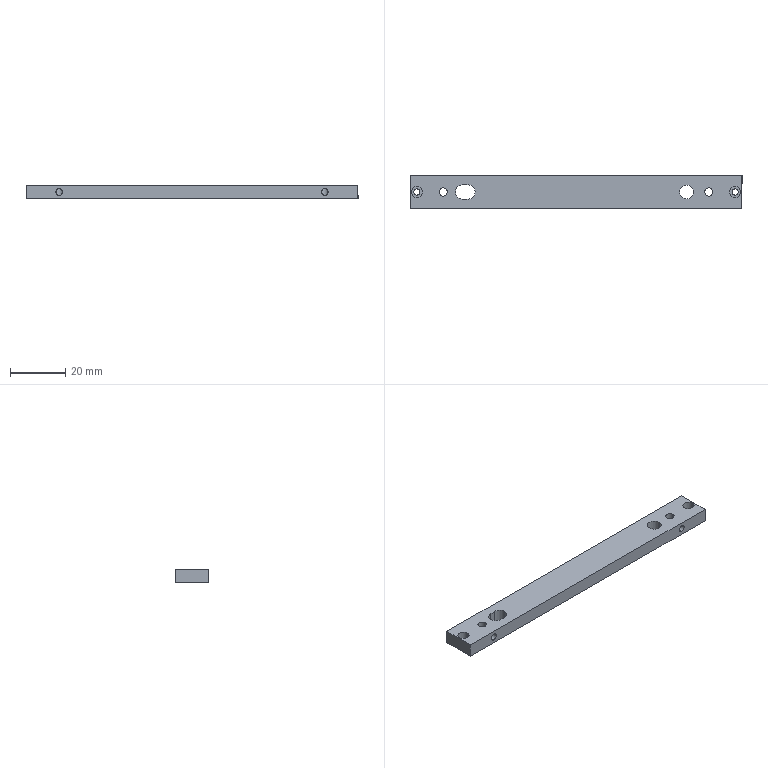Part | SolidWorks | features BaseBody 1 | 1 solid | 35 faces | box 120 x 12 x 5 mm | volume 6743 mm3 | cylinder 21 | plane 10 | cone 4 | commonest cylinder face diameters 2.2 x4 2.459 x4 3 x4 4 x4 5.1 x3 5 x2
STEP:
#1=CARTESIAN_POINT('',(-13.795,0.958,0.));
#2=VERTEX_POINT('',#1);
#3=CARTESIAN_POINT('',(-15.995,0.958,0.));
#4=VERTEX_POINT('',#3);
#5=CARTESIAN_POINT('',(-14.895,0.958,0.));
#6=DIRECTION('',(0.,0.,-1.));
#7=DIRECTION('',(1.,0.,0.));
#8=AXIS2_PLACEMENT_3D('',#5,#6,#7);
#9=CIRCLE('',#8,1.1);
#10=EDGE_CURVE('',#2,#4,#9,.T.);
#11=ORIENTED_EDGE('',*,*,#10,.T.);
#12=CARTESIAN_POINT('',(-15.995,0.958,2.));
#13=VERTEX_POINT('',#12);
#14=CARTESIAN_POINT('',(-15.995,0.958,-115.702));
#15=DIRECTION('',(0.,0.,1.));
#16=VECTOR('',#15,1000.);
#17=LINE('',#14,#16);
#18=EDGE_CURVE('',#4,#13,#17,.T.);
#19=ORIENTED_EDGE('',*,*,#18,.T.);
#20=CARTESIAN_POINT('',(-13.795,0.958,2.));
#21=VERTEX_POINT('',#20);
#22=CARTESIAN_POINT('',(-14.895,0.958,2.));
#23=DIRECTION('',(0.,0.,-1.));
#24=DIRECTION('',(1.,0.,0.));
#25=AXIS2_PLACEMENT_3D('',#22,#23,#24);
#26=CIRCLE('',#25,1.1);
#27=EDGE_CURVE('',#21,#13,#26,.T.);
#28=ORIENTED_EDGE('',*,*,#27,.F.);
#29=CARTESIAN_POINT('',(-13.795,0.958,-115.702));
#30=DIRECTION('',(0.,0.,1.));
#31=VECTOR('',#30,1000.);
#32=LINE('',#29,#31);
#33=EDGE_CURVE('',#2,#21,#32,.T.);
#34=ORIENTED_EDGE('',*,*,#33,.F.);
#35=EDGE_LOOP('',(#11,#19,#28,#34));
#36=FACE_OUTER_BOUND('',#35,.T.);
#37=CARTESIAN_POINT('',(-14.895,0.958,-115.702));
#38=DIRECTION('',(0.,0.,1.));
#39=DIRECTION('',(1.,0.,0.));
#40=AXIS2_PLACEMENT_3D('',#37,#38,#39);
#41=CYLINDRICAL_SURFACE('',#40,1.1);
#42=ADVANCED_FACE('',(#36),#41,.F.);
#43=CARTESIAN_POINT('',(101.205,0.958,0.));
#44=VERTEX_POINT('',#43);
#45=CARTESIAN_POINT('',(99.005,0.958,0.));
#46=VERTEX_POINT('',#45);
#47=CARTESIAN_POINT('',(100.105,0.958,0.));
#48=DIRECTION('',(0.,0.,-1.));
#49=DIRECTION('',(1.,0.,0.));
#50=AXIS2_PLACEMENT_3D('',#47,#48,#49);
#51=CIRCLE('',#50,1.1);
#52=EDGE_CURVE('',#44,#46,#51,.T.);
#53=ORIENTED_EDGE('',*,*,#52,.T.);
#54=CARTESIAN_POINT('',(99.005,0.958,2.));
#55=VERTEX_POINT('',#54);
#56=CARTESIAN_POINT('',(99.005,0.958,-115.702));
#57=DIRECTION('',(0.,0.,1.));
#58=VECTOR('',#57,1000.);
#59=LINE('',#56,#58);
#60=EDGE_CURVE('',#46,#55,#59,.T.);
#61=ORIENTED_EDGE('',*,*,#60,.T.);
#62=CARTESIAN_POINT('',(101.205,0.958,2.));
#63=VERTEX_POINT('',#62);
#64=CARTESIAN_POINT('',(100.105,0.958,2.));
#65=DIRECTION('',(0.,0.,-1.));
#66=DIRECTION('',(1.,0.,0.));
#67=AXIS2_PLACEMENT_3D('',#64,#65,#66);
#68=CIRCLE('',#67,1.1);
#69=EDGE_CURVE('',#63,#55,#68,.T.);
#70=ORIENTED_EDGE('',*,*,#69,.F.);
#71=CARTESIAN_POINT('',(101.205,0.958,-115.702));
#72=DIRECTION('',(0.,0.,1.));
#73=VECTOR('',#72,1000.);
#74=LINE('',#71,#73);
#75=EDGE_CURVE('',#44,#63,#74,.T.);
#76=ORIENTED_EDGE('',*,*,#75,.F.);
#77=EDGE_LOOP('',(#53,#61,#70,#76));
#78=FACE_OUTER_BOUND('',#77,.T.);
#79=CARTESIAN_POINT('',(100.105,0.958,-115.702));
#80=DIRECTION('',(0.,0.,1.));
#81=DIRECTION('',(1.,0.,0.));
#82=AXIS2_PLACEMENT_3D('',#79,#80,#81);
#83=CYLINDRICAL_SURFACE('',#82,1.1);
#84=ADVANCED_FACE('',(#78),#83,.F.);
#85=CARTESIAN_POINT('',(-4.277,-0.04202,1.988));
#86=VERTEX_POINT('',#85);
#87=CARTESIAN_POINT('',(-5.395,-0.542,1.27));
#88=VERTEX_POINT('',#87);
#89=CARTESIAN_POINT('',(-4.277,-0.04202,1.988));
#90=CARTESIAN_POINT('',(-4.325,-0.09543,1.884));
#91=CARTESIAN_POINT('',(-4.384,-0.1541,1.791));
#92=CARTESIAN_POINT('',(-4.528,-0.2694,1.621));
#93=CARTESIAN_POINT('',(-4.612,-0.3262,1.545));
#94=CARTESIAN_POINT('',(-4.802,-0.424,1.417));
#95=CARTESIAN_POINT('',(-4.91,-0.4666,1.364));
#96=CARTESIAN_POINT('',(-5.143,-0.5256,1.29));
#97=CARTESIAN_POINT('',(-5.27,-0.542,1.27));
#98=CARTESIAN_POINT('',(-5.395,-0.542,1.27));
#99=B_SPLINE_CURVE_WITH_KNOTS('',3,(#89,#90,#91,#92,#93,#94,#95,#96,#97,#98),.UNSPECIFIED.,.F.,.F.,(4,2,2,2,4),(0.,0.0003744,0.0007489,0.001123,0.001498),.UNSPECIFIED.);
#100=EDGE_CURVE('',#86,#88,#99,.T.);
#101=ORIENTED_EDGE('',*,*,#100,.F.);
#102=CARTESIAN_POINT('',(-4.277,-0.04202,3.012));
#103=VERTEX_POINT('',#102);
#104=CARTESIAN_POINT('',(-4.277,-0.04202,3.012));
#105=CARTESIAN_POINT('',(-4.252,-0.01371,2.843));
#106=CARTESIAN_POINT('',(-4.239,0.002052,2.673));
#107=CARTESIAN_POINT('',(-4.239,0.002227,2.33));
#108=CARTESIAN_POINT('',(-4.252,-0.01369,2.157));
#109=CARTESIAN_POINT('',(-4.277,-0.04202,1.988));
#110=B_SPLINE_CURVE_WITH_KNOTS('',3,(#104,#105,#106,#107,#108,#109),.UNSPECIFIED.,.F.,.F.,(4,2,4),(0.,0.0005131,0.001026),.UNSPECIFIED.);
#111=EDGE_CURVE('',#103,#86,#110,.T.);
#112=ORIENTED_EDGE('',*,*,#111,.F.);
#113=CARTESIAN_POINT('',(-5.395,-0.542,3.73));
#114=VERTEX_POINT('',#113);
#115=CARTESIAN_POINT('',(-5.395,-0.542,3.73));
#116=CARTESIAN_POINT('',(-5.27,-0.542,3.73));
#117=CARTESIAN_POINT('',(-5.144,-0.5258,3.71));
#118=CARTESIAN_POINT('',(-4.912,-0.4673,3.637));
#119=CARTESIAN_POINT('',(-4.804,-0.4249,3.584));
#120=CARTESIAN_POINT('',(-4.613,-0.3265,3.456));
#121=CARTESIAN_POINT('',(-4.529,-0.2699,3.379));
#122=CARTESIAN_POINT('',(-4.385,-0.1549,3.21));
#123=CARTESIAN_POINT('',(-4.325,-0.09524,3.116));
#124=CARTESIAN_POINT('',(-4.277,-0.04202,3.012));
#125=B_SPLINE_CURVE_WITH_KNOTS('',3,(#115,#116,#117,#118,#119,#120,#121,#122,#123,#124),.UNSPECIFIED.,.F.,.F.,(4,2,2,2,4),(0.001498,0.00187,0.002243,0.002616,0.002988),.UNSPECIFIED.);
#126=EDGE_CURVE('',#114,#103,#125,.T.);
#127=ORIENTED_EDGE('',*,*,#126,.F.);
#128=CARTESIAN_POINT('',(-6.513,-0.04202,3.012));
#129=VERTEX_POINT('',#128);
#130=CARTESIAN_POINT('',(-6.513,-0.04202,3.012));
#131=CARTESIAN_POINT('',(-6.465,-0.09543,3.116));
#132=CARTESIAN_POINT('',(-6.406,-0.1541,3.209));
#133=CARTESIAN_POINT('',(-6.262,-0.2694,3.379));
#134=CARTESIAN_POINT('',(-6.177,-0.3262,3.455));
#135=CARTESIAN_POINT('',(-5.988,-0.424,3.583));
#136=CARTESIAN_POINT('',(-5.88,-0.4666,3.636));
#137=CARTESIAN_POINT('',(-5.647,-0.5256,3.71));
#138=CARTESIAN_POINT('',(-5.52,-0.542,3.729));
#139=CARTESIAN_POINT('',(-5.395,-0.542,3.73));
#140=B_SPLINE_CURVE_WITH_KNOTS('',3,(#130,#131,#132,#133,#134,#135,#136,#137,#138,#139),.UNSPECIFIED.,.F.,.F.,(4,2,2,2,4),(0.,0.0003744,0.0007489,0.001123,0.001498),.UNSPECIFIED.);
#141=EDGE_CURVE('',#129,#114,#140,.T.);
#142=ORIENTED_EDGE('',*,*,#141,.F.);
#143=CARTESIAN_POINT('',(-6.513,-0.04202,1.988));
#144=VERTEX_POINT('',#143);
#145=CARTESIAN_POINT('',(-6.513,-0.04202,1.988));
#146=CARTESIAN_POINT('',(-6.538,-0.01371,2.157));
#147=CARTESIAN_POINT('',(-6.551,0.002052,2.327));
#148=CARTESIAN_POINT('',(-6.551,0.002227,2.67));
#149=CARTESIAN_POINT('',(-6.538,-0.01369,2.843));
#150=CARTESIAN_POINT('',(-6.513,-0.04202,3.012));
#151=B_SPLINE_CURVE_WITH_KNOTS('',3,(#145,#146,#147,#148,#149,#150),.UNSPECIFIED.,.F.,.F.,(4,2,4),(0.,0.0005131,0.001026),.UNSPECIFIED.);
#152=EDGE_CURVE('',#144,#129,#151,.T.);
#153=ORIENTED_EDGE('',*,*,#152,.F.);
#154=CARTESIAN_POINT('',(-5.395,-0.542,1.27));
#155=CARTESIAN_POINT('',(-5.52,-0.542,1.27));
#156=CARTESIAN_POINT('',(-5.646,-0.5258,1.29));
#157=CARTESIAN_POINT('',(-5.878,-0.4673,1.363));
#158=CARTESIAN_POINT('',(-5.986,-0.4249,1.416));
#159=CARTESIAN_POINT('',(-6.177,-0.3265,1.544));
#160=CARTESIAN_POINT('',(-6.261,-0.2699,1.621));
#161=CARTESIAN_POINT('',(-6.405,-0.1549,1.79));
#162=CARTESIAN_POINT('',(-6.465,-0.09524,1.884));
#163=CARTESIAN_POINT('',(-6.513,-0.04202,1.988));
#164=B_SPLINE_CURVE_WITH_KNOTS('',3,(#154,#155,#156,#157,#158,#159,#160,#161,#162,#163),.UNSPECIFIED.,.F.,.F.,(4,2,2,2,4),(0.001498,0.00187,0.002243,0.002616,0.002988),.UNSPECIFIED.);
#165=EDGE_CURVE('',#88,#144,#164,.T.);
#166=ORIENTED_EDGE('',*,*,#165,.F.);
#167=EDGE_LOOP('',(#101,#112,#127,#142,#153,#166));
#168=FACE_BOUND('',#167,.T.);
#169=CARTESIAN_POINT('',(-3.895,0.958,0.));
#170=VERTEX_POINT('',#169);
#171=CARTESIAN_POINT('',(-6.895,0.958,0.));
#172=VERTEX_POINT('',#171);
#173=CARTESIAN_POINT('',(-5.395,0.958,0.));
#174=DIRECTION('',(0.,0.,-1.));
#175=DIRECTION('',(1.,0.,0.));
#176=AXIS2_PLACEMENT_3D('',#173,#174,#175);
#177=CIRCLE('',#176,1.5);
#178=EDGE_CURVE('',#170,#172,#177,.T.);
#179=ORIENTED_EDGE('',*,*,#178,.T.);
#180=CARTESIAN_POINT('',(-6.895,0.958,5.));
#181=VERTEX_POINT('',#180);
#182=CARTESIAN_POINT('',(-6.895,0.958,-115.702));
#183=DIRECTION('',(0.,0.,1.));
#184=VECTOR('',#183,1000.);
#185=LINE('',#182,#184);
#186=EDGE_CURVE('',#172,#181,#185,.T.);
#187=ORIENTED_EDGE('',*,*,#186,.T.);
#188=CARTESIAN_POINT('',(-3.895,0.958,5.));
#189=VERTEX_POINT('',#188);
#190=CARTESIAN_POINT('',(-5.395,0.958,5.));
#191=DIRECTION('',(0.,0.,-1.));
#192=DIRECTION('',(1.,0.,0.));
#193=AXIS2_PLACEMENT_3D('',#190,#191,#192);
#194=CIRCLE('',#193,1.5);
#195=EDGE_CURVE('',#189,#181,#194,.T.);
#196=ORIENTED_EDGE('',*,*,#195,.F.);
#197=CARTESIAN_POINT('',(-3.895,0.958,-115.702));
#198=DIRECTION('',(0.,0.,1.));
#199=VECTOR('',#198,1000.);
#200=LINE('',#197,#199);
#201=EDGE_CURVE('',#170,#189,#200,.T.);
#202=ORIENTED_EDGE('',*,*,#201,.F.);
#203=EDGE_LOOP('',(#179,#187,#196,#202));
#204=FACE_OUTER_BOUND('',#203,.T.);
#205=CARTESIAN_POINT('',(-5.395,0.958,-115.702));
#206=DIRECTION('',(0.,0.,1.));
#207=DIRECTION('',(1.,0.,0.));
#208=AXIS2_PLACEMENT_3D('',#205,#206,#207);
#209=CYLINDRICAL_SURFACE('',#208,1.5);
#210=ADVANCED_FACE('',(#168,#204),#209,.F.);
#211=CARTESIAN_POINT('',(91.723,-0.04202,1.988));
#212=VERTEX_POINT('',#211);
#213=CARTESIAN_POINT('',(90.605,-0.542,1.27));
#214=VERTEX_POINT('',#213);
#215=CARTESIAN_POINT('',(91.723,-0.04202,1.988));
#216=CARTESIAN_POINT('',(91.675,-0.09543,1.884));
#217=CARTESIAN_POINT('',(91.616,-0.1541,1.791));
#218=CARTESIAN_POINT('',(91.472,-0.2694,1.621));
#219=CARTESIAN_POINT('',(91.388,-0.3262,1.545));
#220=CARTESIAN_POINT('',(91.198,-0.424,1.417));
#221=CARTESIAN_POINT('',(91.09,-0.4666,1.364));
#222=CARTESIAN_POINT('',(90.857,-0.5256,1.29));
#223=CARTESIAN_POINT('',(90.73,-0.542,1.27));
#224=CARTESIAN_POINT('',(90.605,-0.542,1.27));
#225=B_SPLINE_CURVE_WITH_KNOTS('',3,(#215,#216,#217,#218,#219,#220,#221,#222,#223,#224),.UNSPECIFIED.,.F.,.F.,(4,2,2,2,4),(0.,0.0003744,0.0007489,0.001123,0.001498),.UNSPECIFIED.);
#226=EDGE_CURVE('',#212,#214,#225,.T.);
#227=ORIENTED_EDGE('',*,*,#226,.F.);
#228=CARTESIAN_POINT('',(91.723,-0.04202,3.012));
#229=VERTEX_POINT('',#228);
#230=CARTESIAN_POINT('',(91.723,-0.04202,3.012));
#231=CARTESIAN_POINT('',(91.748,-0.01371,2.843));
#232=CARTESIAN_POINT('',(91.761,0.002052,2.673));
#233=CARTESIAN_POINT('',(91.761,0.002227,2.33));
#234=CARTESIAN_POINT('',(91.748,-0.01369,2.157));
#235=CARTESIAN_POINT('',(91.723,-0.04202,1.988));
#236=B_SPLINE_CURVE_WITH_KNOTS('',3,(#230,#231,#232,#233,#234,#235),.UNSPECIFIED.,.F.,.F.,(4,2,4),(0.,0.0005131,0.001026),.UNSPECIFIED.);
#237=EDGE_CURVE('',#229,#212,#236,.T.);
#238=ORIENTED_EDGE('',*,*,#237,.F.);
#239=CARTESIAN_POINT('',(90.605,-0.542,3.73));
#240=VERTEX_POINT('',#239);
#241=CARTESIAN_POINT('',(90.605,-0.542,3.73));
#242=CARTESIAN_POINT('',(90.73,-0.542,3.729));
#243=CARTESIAN_POINT('',(90.856,-0.5258,3.71));
#244=CARTESIAN_POINT('',(91.088,-0.4673,3.637));
#245=CARTESIAN_POINT('',(91.196,-0.4249,3.584));
#246=CARTESIAN_POINT('',(91.387,-0.3265,3.456));
#247=CARTESIAN_POINT('',(91.471,-0.2699,3.379));
#248=CARTESIAN_POINT('',(91.615,-0.1549,3.21));
#249=CARTESIAN_POINT('',(91.675,-0.09524,3.116));
#250=CARTESIAN_POINT('',(91.723,-0.04202,3.012));
#251=B_SPLINE_CURVE_WITH_KNOTS('',3,(#241,#242,#243,#244,#245,#246,#247,#248,#249,#250),.UNSPECIFIED.,.F.,.F.,(4,2,2,2,4),(0.001498,0.00187,0.002243,0.002616,0.002988),.UNSPECIFIED.);
#252=EDGE_CURVE('',#240,#229,#251,.T.);
#253=ORIENTED_EDGE('',*,*,#252,.F.);
#254=CARTESIAN_POINT('',(89.487,-0.04202,3.012));
#255=VERTEX_POINT('',#254);
#256=CARTESIAN_POINT('',(89.487,-0.04202,3.012));
#257=CARTESIAN_POINT('',(89.535,-0.09543,3.116));
#258=CARTESIAN_POINT('',(89.594,-0.1541,3.209));
#259=CARTESIAN_POINT('',(89.738,-0.2694,3.379));
#260=CARTESIAN_POINT('',(89.823,-0.3262,3.455));
#261=CARTESIAN_POINT('',(90.012,-0.424,3.583));
#262=CARTESIAN_POINT('',(90.12,-0.4666,3.636));
#263=CARTESIAN_POINT('',(90.353,-0.5256,3.71));
#264=CARTESIAN_POINT('',(90.48,-0.542,3.73));
#265=CARTESIAN_POINT('',(90.605,-0.542,3.73));
#266=B_SPLINE_CURVE_WITH_KNOTS('',3,(#256,#257,#258,#259,#260,#261,#262,#263,#264,#265),.UNSPECIFIED.,.F.,.F.,(4,2,2,2,4),(0.,0.0003744,0.0007489,0.001123,0.001498),.UNSPECIFIED.);
#267=EDGE_CURVE('',#255,#240,#266,.T.);
#268=ORIENTED_EDGE('',*,*,#267,.F.);
#269=CARTESIAN_POINT('',(89.487,-0.04202,1.988));
#270=VERTEX_POINT('',#269);
#271=CARTESIAN_POINT('',(89.487,-0.04202,1.988));
#272=CARTESIAN_POINT('',(89.462,-0.01371,2.157));
#273=CARTESIAN_POINT('',(89.449,0.002052,2.327));
#274=CARTESIAN_POINT('',(89.449,0.002227,2.67));
#275=CARTESIAN_POINT('',(89.462,-0.01369,2.843));
#276=CARTESIAN_POINT('',(89.487,-0.04202,3.012));
#277=B_SPLINE_CURVE_WITH_KNOTS('',3,(#271,#272,#273,#274,#275,#276),.UNSPECIFIED.,.F.,.F.,(4,2,4),(0.,0.0005131,0.001026),.UNSPECIFIED.);
#278=EDGE_CURVE('',#270,#255,#277,.T.);
#279=ORIENTED_EDGE('',*,*,#278,.F.);
#280=CARTESIAN_POINT('',(90.605,-0.542,1.27));
#281=CARTESIAN_POINT('',(90.48,-0.542,1.271));
#282=CARTESIAN_POINT('',(90.354,-0.5258,1.29));
#283=CARTESIAN_POINT('',(90.122,-0.4673,1.363));
#284=CARTESIAN_POINT('',(90.014,-0.4249,1.416));
#285=CARTESIAN_POINT('',(89.823,-0.3265,1.544));
#286=CARTESIAN_POINT('',(89.739,-0.2699,1.621));
#287=CARTESIAN_POINT('',(89.595,-0.1549,1.79));
#288=CARTESIAN_POINT('',(89.535,-0.09524,1.884));
#289=CARTESIAN_POINT('',(89.487,-0.04202,1.988));
#290=B_SPLINE_CURVE_WITH_KNOTS('',3,(#280,#281,#282,#283,#284,#285,#286,#287,#288,#289),.UNSPECIFIED.,.F.,.F.,(4,2,2,2,4),(0.001498,0.00187,0.002243,0.002616,0.002988),.UNSPECIFIED.);
#291=EDGE_CURVE('',#214,#270,#290,.T.);
#292=ORIENTED_EDGE('',*,*,#291,.F.);
#293=EDGE_LOOP('',(#227,#238,#253,#268,#279,#292));
#294=FACE_BOUND('',#293,.T.);
#295=CARTESIAN_POINT('',(92.105,0.958,0.));
#296=VERTEX_POINT('',#295);
#297=CARTESIAN_POINT('',(89.105,0.958,0.));
#298=VERTEX_POINT('',#297);
#299=CARTESIAN_POINT('',(90.605,0.958,0.));
#300=DIRECTION('',(0.,0.,-1.));
#301=DIRECTION('',(1.,0.,0.));
#302=AXIS2_PLACEMENT_3D('',#299,#300,#301);
#303=CIRCLE('',#302,1.5);
#304=EDGE_CURVE('',#296,#298,#303,.T.);
#305=ORIENTED_EDGE('',*,*,#304,.T.);
#306=CARTESIAN_POINT('',(89.105,0.958,5.));
#307=VERTEX_POINT('',#306);
#308=CARTESIAN_POINT('',(89.105,0.958,-115.702));
#309=DIRECTION('',(0.,0.,1.));
#310=VECTOR('',#309,1000.);
#311=LINE('',#308,#310);
#312=EDGE_CURVE('',#298,#307,#311,.T.);
#313=ORIENTED_EDGE('',*,*,#312,.T.);
#314=CARTESIAN_POINT('',(92.105,0.958,5.));
#315=VERTEX_POINT('',#314);
#316=CARTESIAN_POINT('',(90.605,0.958,5.));
#317=DIRECTION('',(0.,0.,-1.));
#318=DIRECTION('',(1.,0.,0.));
#319=AXIS2_PLACEMENT_3D('',#316,#317,#318);
#320=CIRCLE('',#319,1.5);
#321=EDGE_CURVE('',#315,#307,#320,.T.);
#322=ORIENTED_EDGE('',*,*,#321,.F.);
#323=CARTESIAN_POINT('',(92.105,0.958,-115.702));
#324=DIRECTION('',(0.,0.,1.));
#325=VECTOR('',#324,1000.);
#326=LINE('',#323,#325);
#327=EDGE_CURVE('',#296,#315,#326,.T.);
#328=ORIENTED_EDGE('',*,*,#327,.F.);
#329=EDGE_LOOP('',(#305,#313,#322,#328));
#330=FACE_OUTER_BOUND('',#329,.T.);
#331=CARTESIAN_POINT('',(90.605,0.958,-115.702));
#332=DIRECTION('',(0.,0.,1.));
#333=DIRECTION('',(1.,0.,0.));
#334=AXIS2_PLACEMENT_3D('',#331,#332,#333);
#335=CYLINDRICAL_SURFACE('',#334,1.5);
#336=ADVANCED_FACE('',(#294,#330),#335,.F.);
#337=CARTESIAN_POINT('',(85.105,0.958,5.));
#338=VERTEX_POINT('',#337);
#339=CARTESIAN_POINT('',(80.105,0.958,5.));
#340=VERTEX_POINT('',#339);
#341=CARTESIAN_POINT('',(82.605,0.958,5.));
#342=DIRECTION('',(0.,0.,-1.));
#343=DIRECTION('',(-1.,0.,0.));
#344=AXIS2_PLACEMENT_3D('',#341,#342,#343);
#345=CIRCLE('',#344,2.5);
#346=EDGE_CURVE('',#338,#340,#345,.T.);
#347=ORIENTED_EDGE('',*,*,#346,.F.);
#348=CARTESIAN_POINT('',(85.105,0.958,0.));
#349=VERTEX_POINT('',#348);
#350=CARTESIAN_POINT('',(85.105,0.958,120.702));
#351=DIRECTION('',(0.,0.,-1.));
#352=VECTOR('',#351,1000.);
#353=LINE('',#350,#352);
#354=EDGE_CURVE('',#338,#349,#353,.T.);
#355=ORIENTED_EDGE('',*,*,#354,.T.);
#356=CARTESIAN_POINT('',(80.105,0.958,0.));
#357=VERTEX_POINT('',#356);
#358=CARTESIAN_POINT('',(82.605,0.958,0.));
#359=DIRECTION('',(0.,0.,-1.));
#360=DIRECTION('',(-1.,0.,0.));
#361=AXIS2_PLACEMENT_3D('',#358,#359,#360);
#362=CIRCLE('',#361,2.5);
#363=EDGE_CURVE('',#349,#357,#362,.T.);
#364=ORIENTED_EDGE('',*,*,#363,.T.);
#365=CARTESIAN_POINT('',(80.105,0.958,120.702));
#366=DIRECTION('',(0.,0.,-1.));
#367=VECTOR('',#366,1000.);
#368=LINE('',#365,#367);
#369=EDGE_CURVE('',#340,#357,#368,.T.);
#370=ORIENTED_EDGE('',*,*,#369,.F.);
#371=EDGE_LOOP('',(#347,#355,#364,#370));
#372=FACE_OUTER_BOUND('',#371,.T.);
#373=CARTESIAN_POINT('',(82.605,0.958,120.702));
#374=DIRECTION('',(0.,0.,-1.));
#375=DIRECTION('',(-1.,0.,0.));
#376=AXIS2_PLACEMENT_3D('',#373,#374,#375);
#377=CYLINDRICAL_SURFACE('',#376,2.5);
#378=ADVANCED_FACE('',(#372),#377,.F.);
#379=CARTESIAN_POINT('',(3.605,3.508,0.));
#380=VERTEX_POINT('',#379);
#381=CARTESIAN_POINT('',(6.155,0.958,0.));
#382=VERTEX_POINT('',#381);
#383=CARTESIAN_POINT('',(3.605,0.958,0.));
#384=DIRECTION('',(0.,0.,-1.));
#385=DIRECTION('',(1.,0.,0.));
#386=AXIS2_PLACEMENT_3D('',#383,#384,#385);
#387=CIRCLE('',#386,2.55);
#388=EDGE_CURVE('',#380,#382,#387,.T.);
#389=ORIENTED_EDGE('',*,*,#388,.T.);
#390=CARTESIAN_POINT('',(6.155,0.958,5.));
#391=VERTEX_POINT('',#390);
#392=CARTESIAN_POINT('',(6.155,0.958,0.));
#393=DIRECTION('',(0.,0.,1.));
#394=VECTOR('',#393,1000.);
#395=LINE('',#392,#394);
#396=EDGE_CURVE('',#382,#391,#395,.T.);
#397=ORIENTED_EDGE('',*,*,#396,.T.);
#398=CARTESIAN_POINT('',(3.605,3.508,5.));
#399=VERTEX_POINT('',#398);
#400=CARTESIAN_POINT('',(3.605,0.958,5.));
#401=DIRECTION('',(0.,0.,-1.));
#402=DIRECTION('',(1.,0.,0.));
#403=AXIS2_PLACEMENT_3D('',#400,#401,#402);
#404=CIRCLE('',#403,2.55);
#405=EDGE_CURVE('',#399,#391,#404,.T.);
#406=ORIENTED_EDGE('',*,*,#405,.F.);
#407=CARTESIAN_POINT('',(3.605,3.508,0.));
#408=DIRECTION('',(0.,0.,1.));
#409=VECTOR('',#408,1000.);
#410=LINE('',#407,#409);
#411=EDGE_CURVE('',#380,#399,#410,.T.);
#412=ORIENTED_EDGE('',*,*,#411,.F.);
#413=EDGE_LOOP('',(#389,#397,#406,#412));
#414=FACE_OUTER_BOUND('',#413,.T.);
#415=CARTESIAN_POINT('',(3.605,0.958,0.));
#416=DIRECTION('',(0.,0.,1.));
#417=DIRECTION('',(1.,0.,0.));
#418=AXIS2_PLACEMENT_3D('',#415,#416,#417);
#419=CYLINDRICAL_SURFACE('',#418,2.55);
#420=ADVANCED_FACE('',(#414),#419,.F.);
#421=ORIENTED_EDGE('',*,*,#141,.T.);
#422=CARTESIAN_POINT('',(-5.395,-5.042,3.73));
#423=VERTEX_POINT('',#422);
#424=CARTESIAN_POINT('',(-5.395,-2.542,3.73));
#425=DIRECTION('',(0.,-1.,0.));
#426=VECTOR('',#425,1000.);
#427=LINE('',#424,#426);
#428=EDGE_CURVE('',#114,#423,#427,.T.);
#429=ORIENTED_EDGE('',*,*,#428,.T.);
#430=CARTESIAN_POINT('',(-5.395,-5.042,1.27));
#431=VERTEX_POINT('',#430);
#432=CARTESIAN_POINT('',(-5.395,-5.042,2.5));
#433=DIRECTION('',(0.,1.,0.));
#434=DIRECTION('',(0.,0.,-1.));
#435=AXIS2_PLACEMENT_3D('',#432,#433,#434);
#436=CIRCLE('',#435,1.23);
#437=EDGE_CURVE('',#431,#423,#436,.T.);
#438=ORIENTED_EDGE('',*,*,#437,.F.);
#439=CARTESIAN_POINT('',(-5.395,-2.542,1.27));
#440=DIRECTION('',(0.,-1.,0.));
#441=VECTOR('',#440,1000.);
#442=LINE('',#439,#441);
#443=EDGE_CURVE('',#88,#431,#442,.T.);
#444=ORIENTED_EDGE('',*,*,#443,.F.);
#445=ORIENTED_EDGE('',*,*,#165,.T.);
#446=CARTESIAN_POINT('',(-5.395,-0.04202,2.5));
#447=DIRECTION('',(0.,1.,0.));
#448=DIRECTION('',(1.,0.,0.));
#449=AXIS2_PLACEMENT_3D('',#446,#447,#448);
#450=CIRCLE('',#449,1.229);
#451=EDGE_CURVE('',#144,#129,#450,.T.);
#452=ORIENTED_EDGE('',*,*,#451,.T.);
#453=EDGE_LOOP('',(#421,#429,#438,#444,#445,#452));
#454=FACE_OUTER_BOUND('',#453,.T.);
#455=CARTESIAN_POINT('',(-5.395,-2.542,2.5));
#456=DIRECTION('',(0.,-1.,0.));
#457=DIRECTION('',(0.,0.,-1.));
#458=AXIS2_PLACEMENT_3D('',#455,#456,#457);
#459=CYLINDRICAL_SURFACE('',#458,1.23);
#460=ADVANCED_FACE('',(#454),#459,.F.);
#461=ORIENTED_EDGE('',*,*,#267,.T.);
#462=CARTESIAN_POINT('',(90.605,-5.042,3.73));
#463=VERTEX_POINT('',#462);
#464=CARTESIAN_POINT('',(90.605,-2.542,3.73));
#465=DIRECTION('',(0.,-1.,0.));
#466=VECTOR('',#465,1000.);
#467=LINE('',#464,#466);
#468=EDGE_CURVE('',#240,#463,#467,.T.);
#469=ORIENTED_EDGE('',*,*,#468,.T.);
#470=CARTESIAN_POINT('',(90.605,-5.042,1.27));
#471=VERTEX_POINT('',#470);
#472=CARTESIAN_POINT('',(90.605,-5.042,2.5));
#473=DIRECTION('',(0.,1.,0.));
#474=DIRECTION('',(0.,0.,-1.));
#475=AXIS2_PLACEMENT_3D('',#472,#473,#474);
#476=CIRCLE('',#475,1.23);
#477=EDGE_CURVE('',#471,#463,#476,.T.);
#478=ORIENTED_EDGE('',*,*,#477,.F.);
#479=CARTESIAN_POINT('',(90.605,-2.542,1.27));
#480=DIRECTION('',(0.,-1.,0.));
#481=VECTOR('',#480,1000.);
#482=LINE('',#479,#481);
#483=EDGE_CURVE('',#214,#471,#482,.T.);
#484=ORIENTED_EDGE('',*,*,#483,.F.);
#485=ORIENTED_EDGE('',*,*,#291,.T.);
#486=CARTESIAN_POINT('',(90.605,-0.04202,2.5));
#487=DIRECTION('',(0.,1.,0.));
#488=DIRECTION('',(1.,0.,0.));
#489=AXIS2_PLACEMENT_3D('',#486,#487,#488);
#490=CIRCLE('',#489,1.229);
#491=EDGE_CURVE('',#270,#255,#490,.T.);
#492=ORIENTED_EDGE('',*,*,#491,.T.);
#493=EDGE_LOOP('',(#461,#469,#478,#484,#485,#492));
#494=FACE_OUTER_BOUND('',#493,.T.);
#495=CARTESIAN_POINT('',(90.605,-2.542,2.5));
#496=DIRECTION('',(0.,-1.,0.));
#497=DIRECTION('',(0.,0.,-1.));
#498=AXIS2_PLACEMENT_3D('',#495,#496,#497);
#499=CYLINDRICAL_SURFACE('',#498,1.23);
#500=ADVANCED_FACE('',(#494),#499,.F.);
#501=CARTESIAN_POINT('',(-16.895,0.958,2.));
#502=VERTEX_POINT('',#501);
#503=CARTESIAN_POINT('',(-12.895,0.958,2.));
#504=VERTEX_POINT('',#503);
#505=CARTESIAN_POINT('',(-14.895,0.958,2.));
#506=DIRECTION('',(0.,0.,1.));
#507=DIRECTION('',(1.,0.,0.));
#508=AXIS2_PLACEMENT_3D('',#505,#506,#507);
#509=CIRCLE('',#508,2.);
#510=EDGE_CURVE('',#502,#504,#509,.T.);
#511=ORIENTED_EDGE('',*,*,#510,.F.);
#512=CARTESIAN_POINT('',(-16.895,0.958,5.));
#513=VERTEX_POINT('',#512);
#514=CARTESIAN_POINT('',(-16.895,0.958,3.5));
#515=DIRECTION('',(0.,0.,1.));
#516=VECTOR('',#515,1000.);
#517=LINE('',#514,#516);
#518=EDGE_CURVE('',#502,#513,#517,.T.);
#519=ORIENTED_EDGE('',*,*,#518,.T.);
#520=CARTESIAN_POINT('',(-12.895,0.958,5.));
#521=VERTEX_POINT('',#520);
#522=CARTESIAN_POINT('',(-14.895,0.958,5.));
#523=DIRECTION('',(0.,0.,-1.));
#524=DIRECTION('',(1.,0.,0.));
#525=AXIS2_PLACEMENT_3D('',#522,#523,#524);
#526=CIRCLE('',#525,2.);
#527=EDGE_CURVE('',#521,#513,#526,.T.);
#528=ORIENTED_EDGE('',*,*,#527,.F.);
#529=CARTESIAN_POINT('',(-12.895,0.958,3.5));
#530=DIRECTION('',(0.,0.,1.));
#531=VECTOR('',#530,1000.);
#532=LINE('',#529,#531);
#533=EDGE_CURVE('',#504,#521,#532,.T.);
#534=ORIENTED_EDGE('',*,*,#533,.F.);
#535=EDGE_LOOP('',(#511,#519,#528,#534));
#536=FACE_OUTER_BOUND('',#535,.T.);
#537=CARTESIAN_POINT('',(-14.895,0.958,3.5));
#538=DIRECTION('',(0.,0.,1.));
#539=DIRECTION('',(1.,0.,0.));
#540=AXIS2_PLACEMENT_3D('',#537,#538,#539);
#541=CYLINDRICAL_SURFACE('',#540,2.);
#542=ADVANCED_FACE('',(#536),#541,.F.);
#543=CARTESIAN_POINT('',(98.105,0.958,2.));
#544=VERTEX_POINT('',#543);
#545=CARTESIAN_POINT('',(102.105,0.958,2.));
#546=VERTEX_POINT('',#545);
#547=CARTESIAN_POINT('',(100.105,0.958,2.));
#548=DIRECTION('',(0.,0.,1.));
#549=DIRECTION('',(1.,0.,0.));
#550=AXIS2_PLACEMENT_3D('',#547,#548,#549);
#551=CIRCLE('',#550,2.);
#552=EDGE_CURVE('',#544,#546,#551,.T.);
#553=ORIENTED_EDGE('',*,*,#552,.F.);
#554=CARTESIAN_POINT('',(98.105,0.958,5.));
#555=VERTEX_POINT('',#554);
#556=CARTESIAN_POINT('',(98.105,0.958,3.5));
#557=DIRECTION('',(0.,0.,1.));
#558=VECTOR('',#557,1000.);
#559=LINE('',#556,#558);
#560=EDGE_CURVE('',#544,#555,#559,.T.);
#561=ORIENTED_EDGE('',*,*,#560,.T.);
#562=CARTESIAN_POINT('',(102.105,0.958,5.));
#563=VERTEX_POINT('',#562);
#564=CARTESIAN_POINT('',(100.105,0.958,5.));
#565=DIRECTION('',(0.,0.,-1.));
#566=DIRECTION('',(1.,0.,0.));
#567=AXIS2_PLACEMENT_3D('',#564,#565,#566);
#568=CIRCLE('',#567,2.);
#569=EDGE_CURVE('',#563,#555,#568,.T.);
#570=ORIENTED_EDGE('',*,*,#569,.F.);
#571=CARTESIAN_POINT('',(102.105,0.958,3.5));
#572=DIRECTION('',(0.,0.,1.));
#573=VECTOR('',#572,1000.);
#574=LINE('',#571,#573);
#575=EDGE_CURVE('',#546,#563,#574,.T.);
#576=ORIENTED_EDGE('',*,*,#575,.F.);
#577=EDGE_LOOP('',(#553,#561,#570,#576));
#578=FACE_OUTER_BOUND('',#577,.T.);
#579=CARTESIAN_POINT('',(100.105,0.958,3.5));
#580=DIRECTION('',(0.,0.,1.));
#581=DIRECTION('',(1.,0.,0.));
#582=AXIS2_PLACEMENT_3D('',#579,#580,#581);
#583=CYLINDRICAL_SURFACE('',#582,2.);
#584=ADVANCED_FACE('',(#578),#583,.F.);
#585=ORIENTED_EDGE('',*,*,#10,.F.);
#586=CARTESIAN_POINT('',(-14.895,0.958,0.));
#587=DIRECTION('',(0.,0.,-1.));
#588=DIRECTION('',(1.,0.,0.));
#589=AXIS2_PLACEMENT_3D('',#586,#587,#588);
#590=CIRCLE('',#589,1.1);
#591=EDGE_CURVE('',#4,#2,#590,.T.);
#592=ORIENTED_EDGE('',*,*,#591,.F.);
#593=EDGE_LOOP('',(#585,#592));
#594=FACE_BOUND('',#593,.T.);
#595=ORIENTED_EDGE('',*,*,#52,.F.);
#596=CARTESIAN_POINT('',(100.105,0.958,0.));
#597=DIRECTION('',(0.,0.,-1.));
#598=DIRECTION('',(1.,0.,0.));
#599=AXIS2_PLACEMENT_3D('',#596,#597,#598);
#600=CIRCLE('',#599,1.1);
#601=EDGE_CURVE('',#46,#44,#600,.T.);
#602=ORIENTED_EDGE('',*,*,#601,.F.);
#603=EDGE_LOOP('',(#595,#602));
#604=FACE_BOUND('',#603,.T.);
#605=ORIENTED_EDGE('',*,*,#178,.F.);
#606=CARTESIAN_POINT('',(-5.395,0.958,0.));
#607=DIRECTION('',(0.,0.,-1.));
#608=DIRECTION('',(1.,0.,0.));
#609=AXIS2_PLACEMENT_3D('',#606,#607,#608);
#610=CIRCLE('',#609,1.5);
#611=EDGE_CURVE('',#172,#170,#610,.T.);
#612=ORIENTED_EDGE('',*,*,#611,.F.);
#613=EDGE_LOOP('',(#605,#612));
#614=FACE_BOUND('',#613,.T.);
#615=ORIENTED_EDGE('',*,*,#304,.F.);
#616=CARTESIAN_POINT('',(90.605,0.958,0.));
#617=DIRECTION('',(0.,0.,-1.));
#618=DIRECTION('',(1.,0.,0.));
#619=AXIS2_PLACEMENT_3D('',#616,#617,#618);
#620=CIRCLE('',#619,1.5);
#621=EDGE_CURVE('',#298,#296,#620,.T.);
#622=ORIENTED_EDGE('',*,*,#621,.F.);
#623=EDGE_LOOP('',(#615,#622));
#624=FACE_BOUND('',#623,.T.);
#625=CARTESIAN_POINT('',(82.605,0.958,0.));
#626=DIRECTION('',(0.,0.,-1.));
#627=DIRECTION('',(-1.,0.,0.));
#628=AXIS2_PLACEMENT_3D('',#625,#626,#627);
#629=CIRCLE('',#628,2.5);
#630=EDGE_CURVE('',#357,#349,#629,.T.);
#631=ORIENTED_EDGE('',*,*,#630,.F.);
#632=ORIENTED_EDGE('',*,*,#363,.F.);
#633=EDGE_LOOP('',(#631,#632));
#634=FACE_BOUND('',#633,.T.);
#635=CARTESIAN_POINT('',(3.605,-1.592,0.));
#636=VERTEX_POINT('',#635);
#637=CARTESIAN_POINT('',(1.605,-1.592,0.));
#638=VERTEX_POINT('',#637);
#639=CARTESIAN_POINT('',(42.605,-1.592,0.));
#640=DIRECTION('',(-1.,0.,0.));
#641=VECTOR('',#640,1000.);
#642=LINE('',#639,#641);
#643=EDGE_CURVE('',#636,#638,#642,.T.);
#644=ORIENTED_EDGE('',*,*,#643,.F.);
#645=CARTESIAN_POINT('',(3.605,0.958,0.));
#646=DIRECTION('',(0.,0.,-1.));
#647=DIRECTION('',(1.,0.,0.));
#648=AXIS2_PLACEMENT_3D('',#645,#646,#647);
#649=CIRCLE('',#648,2.55);
#650=EDGE_CURVE('',#382,#636,#649,.T.);
#651=ORIENTED_EDGE('',*,*,#650,.F.);
#652=ORIENTED_EDGE('',*,*,#388,.F.);
#653=CARTESIAN_POINT('',(1.605,3.508,0.));
#654=VERTEX_POINT('',#653);
#655=CARTESIAN_POINT('',(42.605,3.508,0.));
#656=DIRECTION('',(1.,0.,0.));
#657=VECTOR('',#656,1000.);
#658=LINE('',#655,#657);
#659=EDGE_CURVE('',#654,#380,#658,.T.);
#660=ORIENTED_EDGE('',*,*,#659,.F.);
#661=CARTESIAN_POINT('',(1.605,0.958,0.));
#662=DIRECTION('',(0.,0.,-1.));
#663=DIRECTION('',(1.,0.,0.));
#664=AXIS2_PLACEMENT_3D('',#661,#662,#663);
#665=CIRCLE('',#664,2.55);
#666=EDGE_CURVE('',#638,#654,#665,.T.);
#667=ORIENTED_EDGE('',*,*,#666,.F.);
#668=EDGE_LOOP('',(#644,#651,#652,#660,#667));
#669=FACE_BOUND('',#668,.T.);
#670=CARTESIAN_POINT('',(102.605,-5.042,0.));
#671=VERTEX_POINT('',#670);
#672=CARTESIAN_POINT('',(102.605,6.958,0.));
#673=VERTEX_POINT('',#672);
#674=CARTESIAN_POINT('',(102.605,0.958,0.));
#675=DIRECTION('',(0.,1.,0.));
#676=VECTOR('',#675,1000.);
#677=LINE('',#674,#676);
#678=EDGE_CURVE('',#671,#673,#677,.T.);
#679=ORIENTED_EDGE('',*,*,#678,.F.);
#680=CARTESIAN_POINT('',(-17.395,-5.042,0.));
#681=VERTEX_POINT('',#680);
#682=CARTESIAN_POINT('',(42.605,-5.042,0.));
#683=DIRECTION('',(1.,0.,0.));
#684=VECTOR('',#683,1000.);
#685=LINE('',#682,#684);
#686=EDGE_CURVE('',#681,#671,#685,.T.);
#687=ORIENTED_EDGE('',*,*,#686,.F.);
#688=CARTESIAN_POINT('',(-17.395,6.958,0.));
#689=VERTEX_POINT('',#688);
#690=CARTESIAN_POINT('',(-17.395,0.958,0.));
#691=DIRECTION('',(0.,-1.,0.));
#692=VECTOR('',#691,1000.);
#693=LINE('',#690,#692);
#694=EDGE_CURVE('',#689,#681,#693,.T.);
#695=ORIENTED_EDGE('',*,*,#694,.F.);
#696=CARTESIAN_POINT('',(42.605,6.958,0.));
#697=DIRECTION('',(-1.,0.,0.));
#698=VECTOR('',#697,1000.);
#699=LINE('',#696,#698);
#700=EDGE_CURVE('',#673,#689,#699,.T.);
#701=ORIENTED_EDGE('',*,*,#700,.F.);
#702=EDGE_LOOP('',(#679,#687,#695,#701));
#703=FACE_OUTER_BOUND('',#702,.T.);
#704=CARTESIAN_POINT('',(42.605,0.958,0.));
#705=DIRECTION('',(0.,0.,1.));
#706=DIRECTION('',(1.,0.,0.));
#707=AXIS2_PLACEMENT_3D('',#704,#705,#706);
#708=PLANE('',#707);
#709=ADVANCED_FACE('',(#594,#604,#614,#624,#634,#669,#703),#708,.F.);
#710=ORIENTED_EDGE('',*,*,#18,.F.);
#711=ORIENTED_EDGE('',*,*,#591,.T.);
#712=ORIENTED_EDGE('',*,*,#33,.T.);
#713=CARTESIAN_POINT('',(-14.895,0.958,2.));
#714=DIRECTION('',(0.,0.,-1.));
#715=DIRECTION('',(1.,0.,0.));
#716=AXIS2_PLACEMENT_3D('',#713,#714,#715);
#717=CIRCLE('',#716,1.1);
#718=EDGE_CURVE('',#13,#21,#717,.T.);
#719=ORIENTED_EDGE('',*,*,#718,.F.);
#720=EDGE_LOOP('',(#710,#711,#712,#719));
#721=FACE_OUTER_BOUND('',#720,.T.);
#722=CARTESIAN_POINT('',(-14.895,0.958,-115.702));
#723=DIRECTION('',(0.,0.,1.));
#724=DIRECTION('',(1.,0.,0.));
#725=AXIS2_PLACEMENT_3D('',#722,#723,#724);
#726=CYLINDRICAL_SURFACE('',#725,1.1);
#727=ADVANCED_FACE('',(#721),#726,.F.);
#728=ORIENTED_EDGE('',*,*,#60,.F.);
#729=ORIENTED_EDGE('',*,*,#601,.T.);
#730=ORIENTED_EDGE('',*,*,#75,.T.);
#731=CARTESIAN_POINT('',(100.105,0.958,2.));
#732=DIRECTION('',(0.,0.,-1.));
#733=DIRECTION('',(1.,0.,0.));
#734=AXIS2_PLACEMENT_3D('',#731,#732,#733);
#735=CIRCLE('',#734,1.1);
#736=EDGE_CURVE('',#55,#63,#735,.T.);
#737=ORIENTED_EDGE('',*,*,#736,.F.);
#738=EDGE_LOOP('',(#728,#729,#730,#737));
#739=FACE_OUTER_BOUND('',#738,.T.);
#740=CARTESIAN_POINT('',(100.105,0.958,-115.702));
#741=DIRECTION('',(0.,0.,1.));
#742=DIRECTION('',(1.,0.,0.));
#743=AXIS2_PLACEMENT_3D('',#740,#741,#742);
#744=CYLINDRICAL_SURFACE('',#743,1.1);
#745=ADVANCED_FACE('',(#739),#744,.F.);
#746=ORIENTED_EDGE('',*,*,#186,.F.);
#747=ORIENTED_EDGE('',*,*,#611,.T.);
#748=ORIENTED_EDGE('',*,*,#201,.T.);
#749=CARTESIAN_POINT('',(-5.395,0.958,5.));
#750=DIRECTION('',(0.,0.,-1.));
#751=DIRECTION('',(1.,0.,0.));
#752=AXIS2_PLACEMENT_3D('',#749,#750,#751);
#753=CIRCLE('',#752,1.5);
#754=EDGE_CURVE('',#181,#189,#753,.T.);
#755=ORIENTED_EDGE('',*,*,#754,.F.);
#756=EDGE_LOOP('',(#746,#747,#748,#755));
#757=FACE_OUTER_BOUND('',#756,.T.);
#758=CARTESIAN_POINT('',(-5.395,0.958,-115.702));
#759=DIRECTION('',(0.,0.,1.));
#760=DIRECTION('',(1.,0.,0.));
#761=AXIS2_PLACEMENT_3D('',#758,#759,#760);
#762=CYLINDRICAL_SURFACE('',#761,1.5);
#763=ADVANCED_FACE('',(#757),#762,.F.);
#764=ORIENTED_EDGE('',*,*,#312,.F.);
#765=ORIENTED_EDGE('',*,*,#621,.T.);
#766=ORIENTED_EDGE('',*,*,#327,.T.);
#767=CARTESIAN_POINT('',(90.605,0.958,5.));
#768=DIRECTION('',(0.,0.,-1.));
#769=DIRECTION('',(1.,0.,0.));
#770=AXIS2_PLACEMENT_3D('',#767,#768,#769);
#771=CIRCLE('',#770,1.5);
#772=EDGE_CURVE('',#307,#315,#771,.T.);
#773=ORIENTED_EDGE('',*,*,#772,.F.);
#774=EDGE_LOOP('',(#764,#765,#766,#773));
#775=FACE_OUTER_BOUND('',#774,.T.);
#776=CARTESIAN_POINT('',(90.605,0.958,-115.702));
#777=DIRECTION('',(0.,0.,1.));
#778=DIRECTION('',(1.,0.,0.));
#779=AXIS2_PLACEMENT_3D('',#776,#777,#778);
#780=CYLINDRICAL_SURFACE('',#779,1.5);
#781=ADVANCED_FACE('',(#775),#780,.F.);
#782=ORIENTED_EDGE('',*,*,#354,.F.);
#783=CARTESIAN_POINT('',(82.605,0.958,5.));
#784=DIRECTION('',(0.,0.,-1.));
#785=DIRECTION('',(-1.,0.,0.));
#786=AXIS2_PLACEMENT_3D('',#783,#784,#785);
#787=CIRCLE('',#786,2.5);
#788=EDGE_CURVE('',#340,#338,#787,.T.);
#789=ORIENTED_EDGE('',*,*,#788,.F.);
#790=ORIENTED_EDGE('',*,*,#369,.T.);
#791=ORIENTED_EDGE('',*,*,#630,.T.);
#792=EDGE_LOOP('',(#782,#789,#790,#791));
#793=FACE_OUTER_BOUND('',#792,.T.);
#794=CARTESIAN_POINT('',(82.605,0.958,120.702));
#795=DIRECTION('',(0.,0.,-1.));
#796=DIRECTION('',(-1.,0.,0.));
#797=AXIS2_PLACEMENT_3D('',#794,#795,#796);
#798=CYLINDRICAL_SURFACE('',#797,2.5);
#799=ADVANCED_FACE('',(#793),#798,.F.);
#800=ORIENTED_EDGE('',*,*,#666,.T.);
#801=CARTESIAN_POINT('',(1.605,3.508,5.));
#802=VERTEX_POINT('',#801);
#803=CARTESIAN_POINT('',(1.605,3.508,0.));
#804=DIRECTION('',(0.,0.,-1.));
#805=VECTOR('',#804,1000.);
#806=LINE('',#803,#805);
#807=EDGE_CURVE('',#802,#654,#806,.T.);
#808=ORIENTED_EDGE('',*,*,#807,.F.);
#809=CARTESIAN_POINT('',(1.605,-1.592,5.));
#810=VERTEX_POINT('',#809);
#811=CARTESIAN_POINT('',(1.605,0.958,5.));
#812=DIRECTION('',(0.,0.,-1.));
#813=DIRECTION('',(1.,0.,0.));
#814=AXIS2_PLACEMENT_3D('',#811,#812,#813);
#815=CIRCLE('',#814,2.55);
#816=EDGE_CURVE('',#810,#802,#815,.T.);
#817=ORIENTED_EDGE('',*,*,#816,.F.);
#818=CARTESIAN_POINT('',(1.605,-1.592,0.));
#819=DIRECTION('',(0.,0.,1.));
#820=VECTOR('',#819,1000.);
#821=LINE('',#818,#820);
#822=EDGE_CURVE('',#638,#810,#821,.T.);
#823=ORIENTED_EDGE('',*,*,#822,.F.);
#824=EDGE_LOOP('',(#800,#808,#817,#823));
#825=FACE_OUTER_BOUND('',#824,.T.);
#826=CARTESIAN_POINT('',(1.605,0.958,0.));
#827=DIRECTION('',(0.,0.,1.));
#828=DIRECTION('',(1.,0.,0.));
#829=AXIS2_PLACEMENT_3D('',#826,#827,#828);
#830=CYLINDRICAL_SURFACE('',#829,2.55);
#831=ADVANCED_FACE('',(#825),#830,.F.);
#832=CARTESIAN_POINT('',(3.605,-1.592,5.));
#833=VERTEX_POINT('',#832);
#834=CARTESIAN_POINT('',(3.605,-1.592,0.));
#835=DIRECTION('',(0.,0.,1.));
#836=VECTOR('',#835,1000.);
#837=LINE('',#834,#836);
#838=EDGE_CURVE('',#636,#833,#837,.T.);
#839=ORIENTED_EDGE('',*,*,#838,.F.);
#840=ORIENTED_EDGE('',*,*,#643,.T.);
#841=ORIENTED_EDGE('',*,*,#822,.T.);
#842=CARTESIAN_POINT('',(3.605,-1.592,5.));
#843=DIRECTION('',(-1.,0.,0.));
#844=VECTOR('',#843,1000.);
#845=LINE('',#842,#844);
#846=EDGE_CURVE('',#833,#810,#845,.T.);
#847=ORIENTED_EDGE('',*,*,#846,.F.);
#848=EDGE_LOOP('',(#839,#840,#841,#847));
#849=FACE_OUTER_BOUND('',#848,.T.);
#850=CARTESIAN_POINT('',(3.605,-1.592,0.));
#851=DIRECTION('',(0.,-1.,0.));
#852=DIRECTION('',(0.,0.,-1.));
#853=AXIS2_PLACEMENT_3D('',#850,#851,#852);
#854=PLANE('',#853);
#855=ADVANCED_FACE('',(#849),#854,.F.);
#856=ORIENTED_EDGE('',*,*,#396,.F.);
#857=ORIENTED_EDGE('',*,*,#650,.T.);
#858=ORIENTED_EDGE('',*,*,#838,.T.);
#859=CARTESIAN_POINT('',(3.605,0.958,5.));
#860=DIRECTION('',(0.,0.,-1.));
#861=DIRECTION('',(1.,0.,0.));
#862=AXIS2_PLACEMENT_3D('',#859,#860,#861);
#863=CIRCLE('',#862,2.55);
#864=EDGE_CURVE('',#391,#833,#863,.T.);
#865=ORIENTED_EDGE('',*,*,#864,.F.);
#866=EDGE_LOOP('',(#856,#857,#858,#865));
#867=FACE_OUTER_BOUND('',#866,.T.);
#868=CARTESIAN_POINT('',(3.605,0.958,0.));
#869=DIRECTION('',(0.,0.,1.));
#870=DIRECTION('',(1.,0.,0.));
#871=AXIS2_PLACEMENT_3D('',#868,#869,#870);
#872=CYLINDRICAL_SURFACE('',#871,2.55);
#873=ADVANCED_FACE('',(#867),#872,.F.);
#874=ORIENTED_EDGE('',*,*,#807,.T.);
#875=ORIENTED_EDGE('',*,*,#659,.T.);
#876=ORIENTED_EDGE('',*,*,#411,.T.);
#877=CARTESIAN_POINT('',(1.605,3.508,5.));
#878=DIRECTION('',(1.,0.,0.));
#879=VECTOR('',#878,1000.);
#880=LINE('',#877,#879);
#881=EDGE_CURVE('',#802,#399,#880,.T.);
#882=ORIENTED_EDGE('',*,*,#881,.F.);
#883=EDGE_LOOP('',(#874,#875,#876,#882));
#884=FACE_OUTER_BOUND('',#883,.T.);
#885=CARTESIAN_POINT('',(1.605,3.508,0.));
#886=DIRECTION('',(0.,1.,0.));
#887=DIRECTION('',(0.,0.,1.));
#888=AXIS2_PLACEMENT_3D('',#885,#886,#887);
#889=PLANE('',#888);
#890=ADVANCED_FACE('',(#884),#889,.F.);
#891=ORIENTED_EDGE('',*,*,#700,.T.);
#892=CARTESIAN_POINT('',(-17.395,6.958,5.));
#893=VERTEX_POINT('',#892);
#894=CARTESIAN_POINT('',(-17.395,6.958,0.));
#895=DIRECTION('',(0.,0.,1.));
#896=VECTOR('',#895,1000.);
#897=LINE('',#894,#896);
#898=EDGE_CURVE('',#689,#893,#897,.T.);
#899=ORIENTED_EDGE('',*,*,#898,.T.);
#900=CARTESIAN_POINT('',(102.605,6.958,5.));
#901=VERTEX_POINT('',#900);
#902=CARTESIAN_POINT('',(-17.395,6.958,5.));
#903=DIRECTION('',(1.,0.,0.));
#904=VECTOR('',#903,1000.);
#905=LINE('',#902,#904);
#906=EDGE_CURVE('',#893,#901,#905,.T.);
#907=ORIENTED_EDGE('',*,*,#906,.T.);
#908=CARTESIAN_POINT('',(102.605,6.958,0.));
#909=DIRECTION('',(0.,0.,-1.));
#910=VECTOR('',#909,1000.);
#911=LINE('',#908,#910);
#912=EDGE_CURVE('',#901,#673,#911,.T.);
#913=ORIENTED_EDGE('',*,*,#912,.T.);
#914=EDGE_LOOP('',(#891,#899,#907,#913));
#915=FACE_OUTER_BOUND('',#914,.T.);
#916=CARTESIAN_POINT('',(-17.395,6.958,0.));
#917=DIRECTION('',(0.,1.,0.));
#918=DIRECTION('',(0.,0.,1.));
#919=AXIS2_PLACEMENT_3D('',#916,#917,#918);
#920=PLANE('',#919);
#921=ADVANCED_FACE('',(#915),#920,.T.);
#922=ORIENTED_EDGE('',*,*,#678,.T.);
#923=ORIENTED_EDGE('',*,*,#912,.F.);
#924=CARTESIAN_POINT('',(102.605,-5.042,5.));
#925=VERTEX_POINT('',#924);
#926=CARTESIAN_POINT('',(102.605,6.958,5.));
#927=DIRECTION('',(0.,-1.,0.));
#928=VECTOR('',#927,1000.);
#929=LINE('',#926,#928);
#930=EDGE_CURVE('',#901,#925,#929,.T.);
#931=ORIENTED_EDGE('',*,*,#930,.T.);
#932=CARTESIAN_POINT('',(102.605,-5.042,0.));
#933=DIRECTION('',(0.,0.,-1.));
#934=VECTOR('',#933,1000.);
#935=LINE('',#932,#934);
#936=EDGE_CURVE('',#925,#671,#935,.T.);
#937=ORIENTED_EDGE('',*,*,#936,.T.);
#938=EDGE_LOOP('',(#922,#923,#931,#937));
#939=FACE_OUTER_BOUND('',#938,.T.);
#940=CARTESIAN_POINT('',(102.605,6.958,0.));
#941=DIRECTION('',(1.,0.,0.));
#942=DIRECTION('',(0.,0.,-1.));
#943=AXIS2_PLACEMENT_3D('',#940,#941,#942);
#944=PLANE('',#943);
#945=ADVANCED_FACE('',(#939),#944,.T.);
#946=ORIENTED_EDGE('',*,*,#437,.T.);
#947=CARTESIAN_POINT('',(-5.395,-5.042,2.5));
#948=DIRECTION('',(0.,1.,0.));
#949=DIRECTION('',(0.,0.,-1.));
#950=AXIS2_PLACEMENT_3D('',#947,#948,#949);
#951=CIRCLE('',#950,1.23);
#952=EDGE_CURVE('',#423,#431,#951,.T.);
#953=ORIENTED_EDGE('',*,*,#952,.T.);
#954=EDGE_LOOP('',(#946,#953));
#955=FACE_BOUND('',#954,.T.);
#956=ORIENTED_EDGE('',*,*,#477,.T.);
#957=CARTESIAN_POINT('',(90.605,-5.042,2.5));
#958=DIRECTION('',(0.,1.,0.));
#959=DIRECTION('',(0.,0.,-1.));
#960=AXIS2_PLACEMENT_3D('',#957,#958,#959);
#961=CIRCLE('',#960,1.23);
#962=EDGE_CURVE('',#463,#471,#961,.T.);
#963=ORIENTED_EDGE('',*,*,#962,.T.);
#964=EDGE_LOOP('',(#956,#963));
#965=FACE_BOUND('',#964,.T.);
#966=ORIENTED_EDGE('',*,*,#686,.T.);
#967=ORIENTED_EDGE('',*,*,#936,.F.);
#968=CARTESIAN_POINT('',(-17.395,-5.042,5.));
#969=VERTEX_POINT('',#968);
#970=CARTESIAN_POINT('',(102.605,-5.042,5.));
#971=DIRECTION('',(-1.,0.,0.));
#972=VECTOR('',#971,1000.);
#973=LINE('',#970,#972);
#974=EDGE_CURVE('',#925,#969,#973,.T.);
#975=ORIENTED_EDGE('',*,*,#974,.T.);
#976=CARTESIAN_POINT('',(-17.395,-5.042,0.));
#977=DIRECTION('',(0.,0.,-1.));
#978=VECTOR('',#977,1000.);
#979=LINE('',#976,#978);
#980=EDGE_CURVE('',#969,#681,#979,.T.);
#981=ORIENTED_EDGE('',*,*,#980,.T.);
#982=EDGE_LOOP('',(#966,#967,#975,#981));
#983=FACE_OUTER_BOUND('',#982,.T.);
#984=CARTESIAN_POINT('',(102.605,-5.042,0.));
#985=DIRECTION('',(0.,-1.,0.));
#986=DIRECTION('',(0.,0.,-1.));
#987=AXIS2_PLACEMENT_3D('',#984,#985,#986);
#988=PLANE('',#987);
#989=ADVANCED_FACE('',(#955,#965,#983),#988,.T.);
#990=ORIENTED_EDGE('',*,*,#694,.T.);
#991=ORIENTED_EDGE('',*,*,#980,.F.);
#992=CARTESIAN_POINT('',(-17.395,-5.042,5.));
#993=DIRECTION('',(0.,1.,0.));
#994=VECTOR('',#993,1000.);
#995=LINE('',#992,#994);
#996=EDGE_CURVE('',#969,#893,#995,.T.);
#997=ORIENTED_EDGE('',*,*,#996,.T.);
#998=ORIENTED_EDGE('',*,*,#898,.F.);
#999=EDGE_LOOP('',(#990,#991,#997,#998));
#1000=FACE_OUTER_BOUND('',#999,.T.);
#1001=CARTESIAN_POINT('',(-17.395,-5.042,0.));
#1002=DIRECTION('',(-1.,0.,0.));
#1003=DIRECTION('',(0.,0.,1.));
#1004=AXIS2_PLACEMENT_3D('',#1001,#1002,#1003);
#1005=PLANE('',#1004);
#1006=ADVANCED_FACE('',(#1000),#1005,.T.);
#1007=ORIENTED_EDGE('',*,*,#27,.T.);
#1008=ORIENTED_EDGE('',*,*,#718,.T.);
#1009=EDGE_LOOP('',(#1007,#1008));
#1010=FACE_BOUND('',#1009,.T.);
#1011=CARTESIAN_POINT('',(-14.895,0.958,2.));
#1012=DIRECTION('',(0.,0.,1.));
#1013=DIRECTION('',(1.,0.,0.));
#1014=AXIS2_PLACEMENT_3D('',#1011,#1012,#1013);
#1015=CIRCLE('',#1014,2.);
#1016=EDGE_CURVE('',#504,#502,#1015,.T.);
#1017=ORIENTED_EDGE('',*,*,#1016,.T.);
#1018=ORIENTED_EDGE('',*,*,#510,.T.);
#1019=EDGE_LOOP('',(#1017,#1018));
#1020=FACE_OUTER_BOUND('',#1019,.T.);
#1021=CARTESIAN_POINT('',(-14.895,0.958,2.));
#1022=DIRECTION('',(0.,0.,1.));
#1023=DIRECTION('',(1.,0.,0.));
#1024=AXIS2_PLACEMENT_3D('',#1021,#1022,#1023);
#1025=PLANE('',#1024);
#1026=ADVANCED_FACE('',(#1010,#1020),#1025,.T.);
#1027=ORIENTED_EDGE('',*,*,#69,.T.);
#1028=ORIENTED_EDGE('',*,*,#736,.T.);
#1029=EDGE_LOOP('',(#1027,#1028));
#1030=FACE_BOUND('',#1029,.T.);
#1031=CARTESIAN_POINT('',(100.105,0.958,2.));
#1032=DIRECTION('',(0.,0.,1.));
#1033=DIRECTION('',(1.,0.,0.));
#1034=AXIS2_PLACEMENT_3D('',#1031,#1032,#1033);
#1035=CIRCLE('',#1034,2.);
#1036=EDGE_CURVE('',#546,#544,#1035,.T.);
#1037=ORIENTED_EDGE('',*,*,#1036,.T.);
#1038=ORIENTED_EDGE('',*,*,#552,.T.);
#1039=EDGE_LOOP('',(#1037,#1038));
#1040=FACE_OUTER_BOUND('',#1039,.T.);
#1041=CARTESIAN_POINT('',(100.105,0.958,2.));
#1042=DIRECTION('',(0.,0.,1.));
#1043=DIRECTION('',(1.,0.,0.));
#1044=AXIS2_PLACEMENT_3D('',#1041,#1042,#1043);
#1045=PLANE('',#1044);
#1046=ADVANCED_FACE('',(#1030,#1040),#1045,.T.);
#1047=ORIENTED_EDGE('',*,*,#527,.T.);
#1048=CARTESIAN_POINT('',(-14.895,0.958,5.));
#1049=DIRECTION('',(0.,0.,-1.));
#1050=DIRECTION('',(1.,0.,0.));
#1051=AXIS2_PLACEMENT_3D('',#1048,#1049,#1050);
#1052=CIRCLE('',#1051,2.);
#1053=EDGE_CURVE('',#513,#521,#1052,.T.);
#1054=ORIENTED_EDGE('',*,*,#1053,.T.);
#1055=EDGE_LOOP('',(#1047,#1054));
#1056=FACE_BOUND('',#1055,.T.);
#1057=ORIENTED_EDGE('',*,*,#569,.T.);
#1058=CARTESIAN_POINT('',(100.105,0.958,5.));
#1059=DIRECTION('',(0.,0.,-1.));
#1060=DIRECTION('',(1.,0.,0.));
#1061=AXIS2_PLACEMENT_3D('',#1058,#1059,#1060);
#1062=CIRCLE('',#1061,2.);
#1063=EDGE_CURVE('',#555,#563,#1062,.T.);
#1064=ORIENTED_EDGE('',*,*,#1063,.T.);
#1065=EDGE_LOOP('',(#1057,#1064));
#1066=FACE_BOUND('',#1065,.T.);
#1067=ORIENTED_EDGE('',*,*,#195,.T.);
#1068=ORIENTED_EDGE('',*,*,#754,.T.);
#1069=EDGE_LOOP('',(#1067,#1068));
#1070=FACE_BOUND('',#1069,.T.);
#1071=ORIENTED_EDGE('',*,*,#321,.T.);
#1072=ORIENTED_EDGE('',*,*,#772,.T.);
#1073=EDGE_LOOP('',(#1071,#1072));
#1074=FACE_BOUND('',#1073,.T.);
#1075=ORIENTED_EDGE('',*,*,#788,.T.);
#1076=ORIENTED_EDGE('',*,*,#346,.T.);
#1077=EDGE_LOOP('',(#1075,#1076));
#1078=FACE_BOUND('',#1077,.T.);
#1079=ORIENTED_EDGE('',*,*,#405,.T.);
#1080=ORIENTED_EDGE('',*,*,#864,.T.);
#1081=ORIENTED_EDGE('',*,*,#846,.T.);
#1082=ORIENTED_EDGE('',*,*,#816,.T.);
#1083=ORIENTED_EDGE('',*,*,#881,.T.);
#1084=EDGE_LOOP('',(#1079,#1080,#1081,#1082,#1083));
#1085=FACE_BOUND('',#1084,.T.);
#1086=ORIENTED_EDGE('',*,*,#996,.F.);
#1087=ORIENTED_EDGE('',*,*,#974,.F.);
#1088=ORIENTED_EDGE('',*,*,#930,.F.);
#1089=ORIENTED_EDGE('',*,*,#906,.F.);
#1090=EDGE_LOOP('',(#1086,#1087,#1088,#1089));
#1091=FACE_OUTER_BOUND('',#1090,.T.);
#1092=CARTESIAN_POINT('',(42.605,0.958,5.));
#1093=DIRECTION('',(0.,0.,1.));
#1094=DIRECTION('',(1.,0.,0.));
#1095=AXIS2_PLACEMENT_3D('',#1092,#1093,#1094);
#1096=PLANE('',#1095);
#1097=ADVANCED_FACE('',(#1056,#1066,#1070,#1074,#1078,#1085,#1091),#1096,.T.);
#1098=ORIENTED_EDGE('',*,*,#451,.F.);
#1099=ORIENTED_EDGE('',*,*,#152,.T.);
#1100=EDGE_LOOP('',(#1098,#1099));
#1101=FACE_OUTER_BOUND('',#1100,.T.);
#1102=CARTESIAN_POINT('',(-5.395,-0.04202,2.5));
#1103=DIRECTION('',(0.,-1.,0.));
#1104=DIRECTION('',(0.,0.,-1.));
#1105=AXIS2_PLACEMENT_3D('',#1102,#1103,#1104);
#1106=CONICAL_SURFACE('',#1105,1.229,1.03);
#1107=ADVANCED_FACE('',(#1101),#1106,.F.);
#1108=ORIENTED_EDGE('',*,*,#428,.F.);
#1109=ORIENTED_EDGE('',*,*,#126,.T.);
#1110=CARTESIAN_POINT('',(-5.395,-0.04202,2.5));
#1111=DIRECTION('',(0.,-1.,0.));
#1112=DIRECTION('',(0.,0.,-1.));
#1113=AXIS2_PLACEMENT_3D('',#1110,#1111,#1112);
#1114=CIRCLE('',#1113,1.23);
#1115=EDGE_CURVE('',#86,#103,#1114,.T.);
#1116=ORIENTED_EDGE('',*,*,#1115,.F.);
#1117=ORIENTED_EDGE('',*,*,#100,.T.);
#1118=ORIENTED_EDGE('',*,*,#443,.T.);
#1119=ORIENTED_EDGE('',*,*,#952,.F.);
#1120=EDGE_LOOP('',(#1108,#1109,#1116,#1117,#1118,#1119));
#1121=FACE_OUTER_BOUND('',#1120,.T.);
#1122=CARTESIAN_POINT('',(-5.395,-2.542,2.5));
#1123=DIRECTION('',(0.,-1.,0.));
#1124=DIRECTION('',(0.,0.,-1.));
#1125=AXIS2_PLACEMENT_3D('',#1122,#1123,#1124);
#1126=CYLINDRICAL_SURFACE('',#1125,1.23);
#1127=ADVANCED_FACE('',(#1121),#1126,.F.);
#1128=ORIENTED_EDGE('',*,*,#1115,.T.);
#1129=ORIENTED_EDGE('',*,*,#111,.T.);
#1130=EDGE_LOOP('',(#1128,#1129));
#1131=FACE_OUTER_BOUND('',#1130,.T.);
#1132=CARTESIAN_POINT('',(-5.395,-0.04202,2.5));
#1133=DIRECTION('',(0.,-1.,0.));
#1134=DIRECTION('',(0.,0.,-1.));
#1135=AXIS2_PLACEMENT_3D('',#1132,#1133,#1134);
#1136=CONICAL_SURFACE('',#1135,1.229,1.03);
#1137=ADVANCED_FACE('',(#1131),#1136,.F.);
#1138=ORIENTED_EDGE('',*,*,#491,.F.);
#1139=ORIENTED_EDGE('',*,*,#278,.T.);
#1140=EDGE_LOOP('',(#1138,#1139));
#1141=FACE_OUTER_BOUND('',#1140,.T.);
#1142=CARTESIAN_POINT('',(90.605,-0.04202,2.5));
#1143=DIRECTION('',(0.,-1.,0.));
#1144=DIRECTION('',(0.,0.,-1.));
#1145=AXIS2_PLACEMENT_3D('',#1142,#1143,#1144);
#1146=CONICAL_SURFACE('',#1145,1.229,1.03);
#1147=ADVANCED_FACE('',(#1141),#1146,.F.);
#1148=ORIENTED_EDGE('',*,*,#468,.F.);
#1149=ORIENTED_EDGE('',*,*,#252,.T.);
#1150=CARTESIAN_POINT('',(90.605,-0.04202,2.5));
#1151=DIRECTION('',(0.,-1.,0.));
#1152=DIRECTION('',(0.,0.,-1.));
#1153=AXIS2_PLACEMENT_3D('',#1150,#1151,#1152);
#1154=CIRCLE('',#1153,1.23);
#1155=EDGE_CURVE('',#212,#229,#1154,.T.);
#1156=ORIENTED_EDGE('',*,*,#1155,.F.);
#1157=ORIENTED_EDGE('',*,*,#226,.T.);
#1158=ORIENTED_EDGE('',*,*,#483,.T.);
#1159=ORIENTED_EDGE('',*,*,#962,.F.);
#1160=EDGE_LOOP('',(#1148,#1149,#1156,#1157,#1158,#1159));
#1161=FACE_OUTER_BOUND('',#1160,.T.);
#1162=CARTESIAN_POINT('',(90.605,-2.542,2.5));
#1163=DIRECTION('',(0.,-1.,0.));
#1164=DIRECTION('',(0.,0.,-1.));
#1165=AXIS2_PLACEMENT_3D('',#1162,#1163,#1164);
#1166=CYLINDRICAL_SURFACE('',#1165,1.23);
#1167=ADVANCED_FACE('',(#1161),#1166,.F.);
#1168=ORIENTED_EDGE('',*,*,#1155,.T.);
#1169=ORIENTED_EDGE('',*,*,#237,.T.);
#1170=EDGE_LOOP('',(#1168,#1169));
#1171=FACE_OUTER_BOUND('',#1170,.T.);
#1172=CARTESIAN_POINT('',(90.605,-0.04202,2.5));
#1173=DIRECTION('',(0.,-1.,0.));
#1174=DIRECTION('',(0.,0.,-1.));
#1175=AXIS2_PLACEMENT_3D('',#1172,#1173,#1174);
#1176=CONICAL_SURFACE('',#1175,1.229,1.03);
#1177=ADVANCED_FACE('',(#1171),#1176,.F.);
#1178=ORIENTED_EDGE('',*,*,#518,.F.);
#1179=ORIENTED_EDGE('',*,*,#1016,.F.);
#1180=ORIENTED_EDGE('',*,*,#533,.T.);
#1181=ORIENTED_EDGE('',*,*,#1053,.F.);
#1182=EDGE_LOOP('',(#1178,#1179,#1180,#1181));
#1183=FACE_OUTER_BOUND('',#1182,.T.);
#1184=CARTESIAN_POINT('',(-14.895,0.958,3.5));
#1185=DIRECTION('',(0.,0.,1.));
#1186=DIRECTION('',(1.,0.,0.));
#1187=AXIS2_PLACEMENT_3D('',#1184,#1185,#1186);
#1188=CYLINDRICAL_SURFACE('',#1187,2.);
#1189=ADVANCED_FACE('',(#1183),#1188,.F.);
#1190=ORIENTED_EDGE('',*,*,#560,.F.);
#1191=ORIENTED_EDGE('',*,*,#1036,.F.);
#1192=ORIENTED_EDGE('',*,*,#575,.T.);
#1193=ORIENTED_EDGE('',*,*,#1063,.F.);
#1194=EDGE_LOOP('',(#1190,#1191,#1192,#1193));
#1195=FACE_OUTER_BOUND('',#1194,.T.);
#1196=CARTESIAN_POINT('',(100.105,0.958,3.5));
#1197=DIRECTION('',(0.,0.,1.));
#1198=DIRECTION('',(1.,0.,0.));
#1199=AXIS2_PLACEMENT_3D('',#1196,#1197,#1198);
#1200=CYLINDRICAL_SURFACE('',#1199,2.);
#1201=ADVANCED_FACE('',(#1195),#1200,.F.);
#1202=CLOSED_SHELL('',(#42,#84,#210,#336,#378,#420,#460,#500,#542,#584,#709,#727,#745,#763,#781,#799,#831,#855,#873,#890,#921,#945,#989,#1006,#1026,#1046,#1097,#1107,#1127,#1137,#1147,#1167,#1177,#1189,#1201));
#1203=MANIFOLD_SOLID_BREP('',#1202);
#1204=CARTESIAN_POINT('',(0.,0.,0.));
#1205=DIRECTION('',(0.,0.,1.));
#1206=DIRECTION('',(1.,0.,0.));
#1207=AXIS2_PLACEMENT_3D('',#1204,#1205,#1206);
#1208=(LENGTH_UNIT()NAMED_UNIT(*)SI_UNIT(.MILLI.,.METRE.));
#1209=UNCERTAINTY_MEASURE_WITH_UNIT(LENGTH_MEASURE(0.00001),#1208,'','');
#1210=(NAMED_UNIT(*)PLANE_ANGLE_UNIT()SI_UNIT($,.RADIAN.));
#1211=(NAMED_UNIT(*)SI_UNIT($,.STERADIAN.)SOLID_ANGLE_UNIT());
#1212=(GEOMETRIC_REPRESENTATION_CONTEXT(3)GLOBAL_UNCERTAINTY_ASSIGNED_CONTEXT((#1209))GLOBAL_UNIT_ASSIGNED_CONTEXT((#1208,#1210,#1211))REPRESENTATION_CONTEXT('',''));
#1213=ADVANCED_BREP_SHAPE_REPRESENTATION('',(#1203,#1207),#1212);